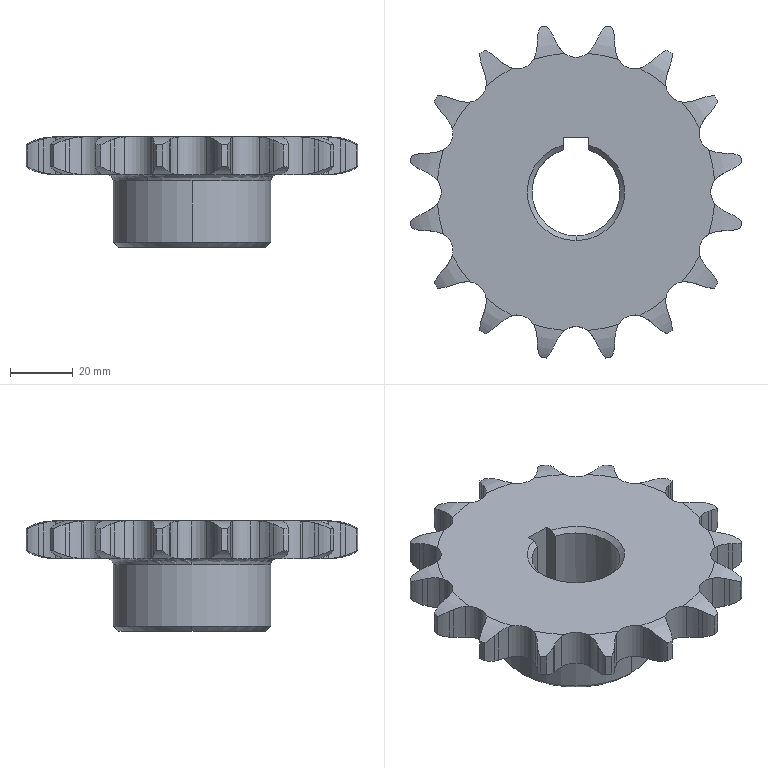Part | SolidWorks | features BaseBody 1 | 1 solid | 183 faces | box 105.504 x 105.504 x 35 mm | volume 103891 mm3 | cylinder 106 | plane 38 | spline 34 | cone 5 | commonest cylinder face diameters 19.857 x34 31.085 x32 12.029 x21 107.201 x16 50 x2 28 x1